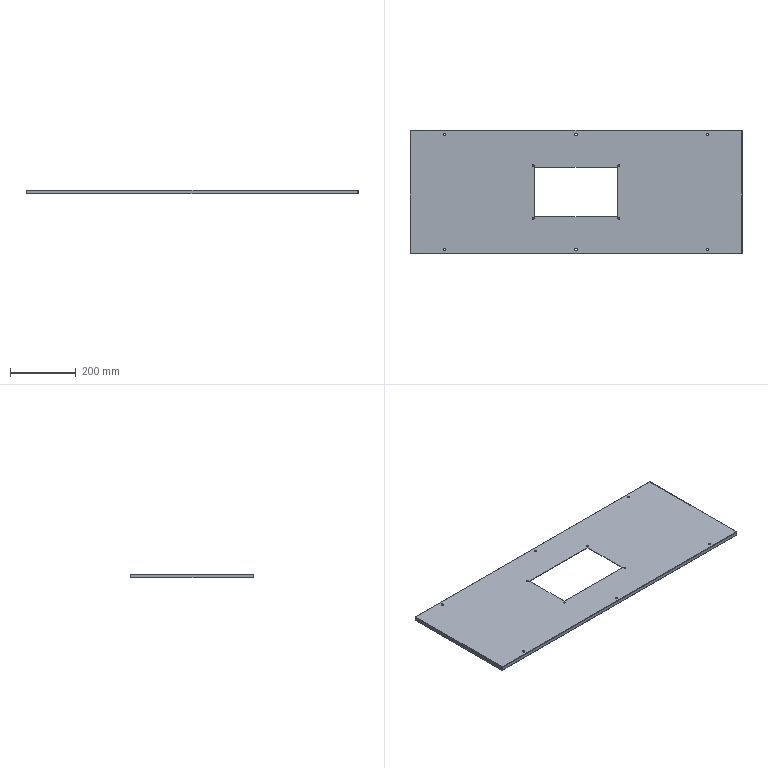Part | SolidWorks | features ICE 2, EdgeFlange 1, FlatPattern 1, SMBaseFlange 1, SheetMetal 1 | 1 solid | 62 faces | box 1010 x 375 x 12 mm | volume 553312 mm3 | cylinder 28 | plane 26 | spline 8 | commonest cylinder face diameters 7 x12 5.1 x8 0.2 x4 3.2 x4